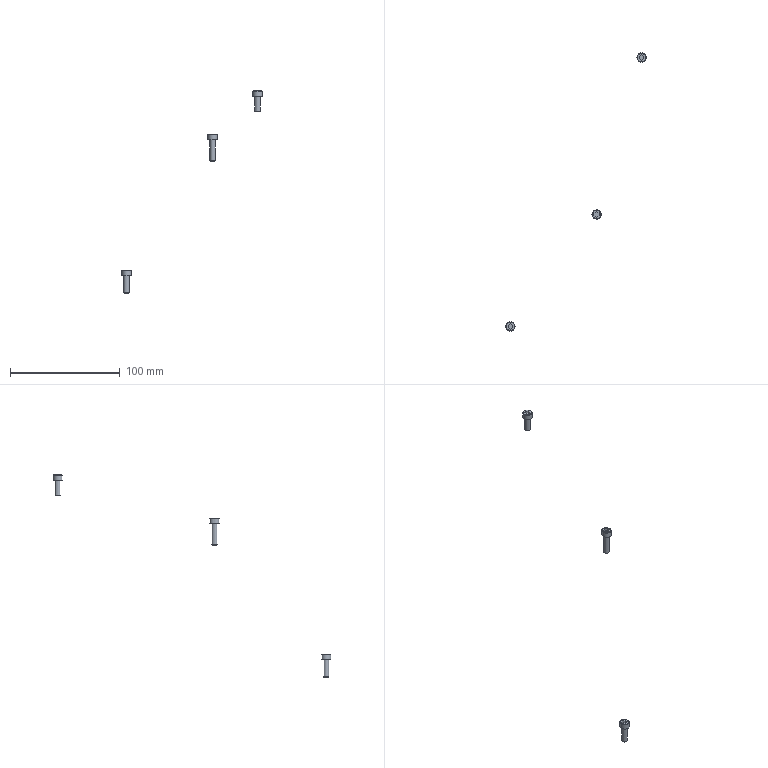Part | STEP file | M5.00-20 | 3 solids | 42 faces | box 128.111 x 253.437 x 184.519 mm | volume 1683 mm3 | plane 30 | cylinder 6 | cone 6 | commonest cylinder face diameters 5 x3 8.5 x3